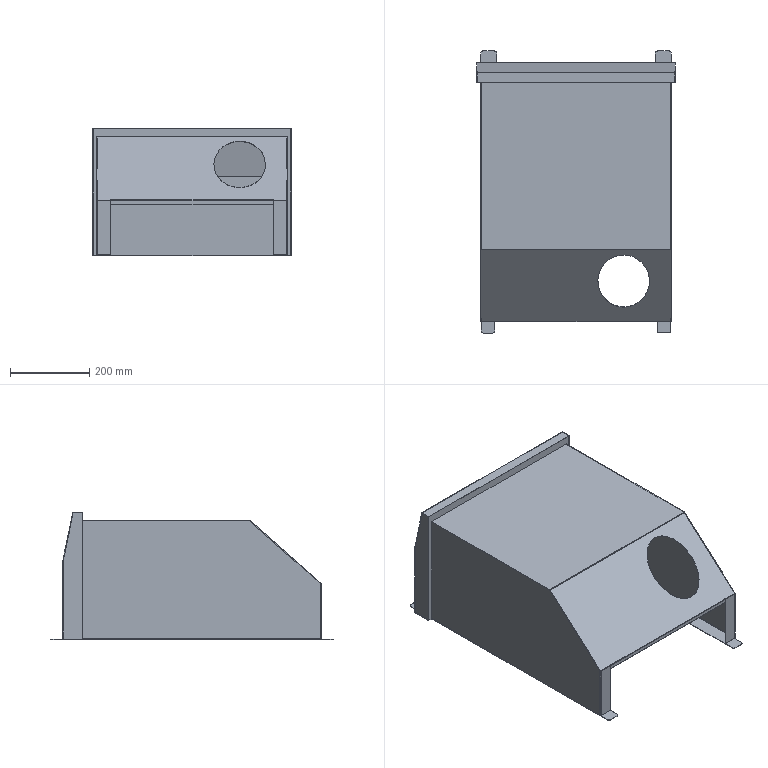Part | SolidWorks | features ICE 6, EdgeFlange 4, Fillet 3, Chamfer 2, SMBaseFlange 2, SheetMetal 2, Cut 1, FlatPattern 1, Shell 1 | 2 solids | 113 faces | box 500 x 710.009 x 320 mm | volume 1088969 mm3 | plane 84 | cylinder 24 | spline 5 | commonest cylinder face diameters 10 x8 1.473 x7 3.873 x7 20 x2